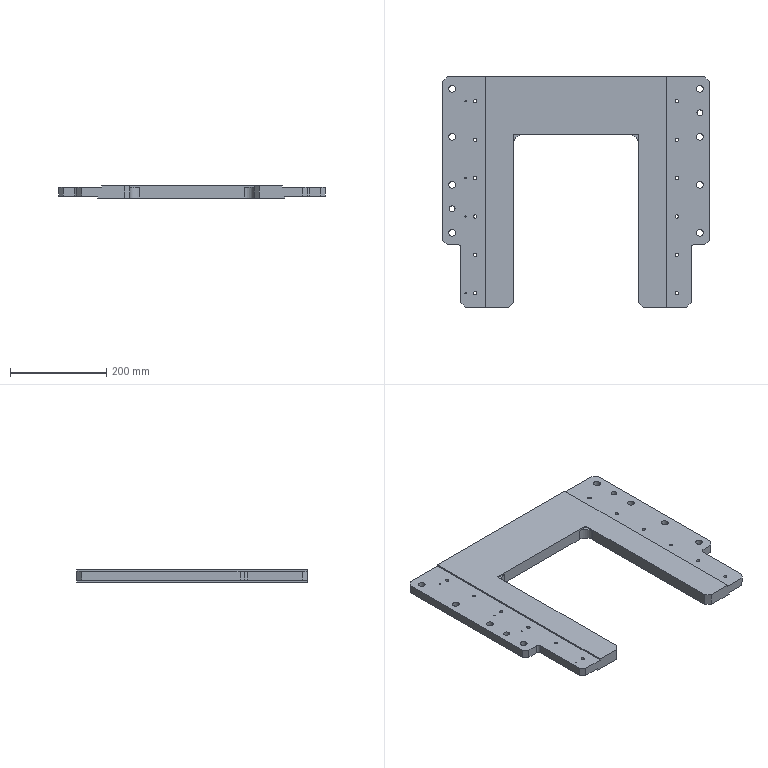Part | SolidWorks | features 3DProfileFeature 5, HoleWzd 5, ICE 3, MirrorPattern 2, Chamfer 1, Extrusion 1, Fillet 1 | 1 solid | 100 faces | box 556 x 480 x 25 mm | volume 3535416 mm3 | cylinder 64 | plane 36 | commonest cylinder face diameters 6.8 x24 14 x16 2.5 x8 7 x8 12 x4 10 x2